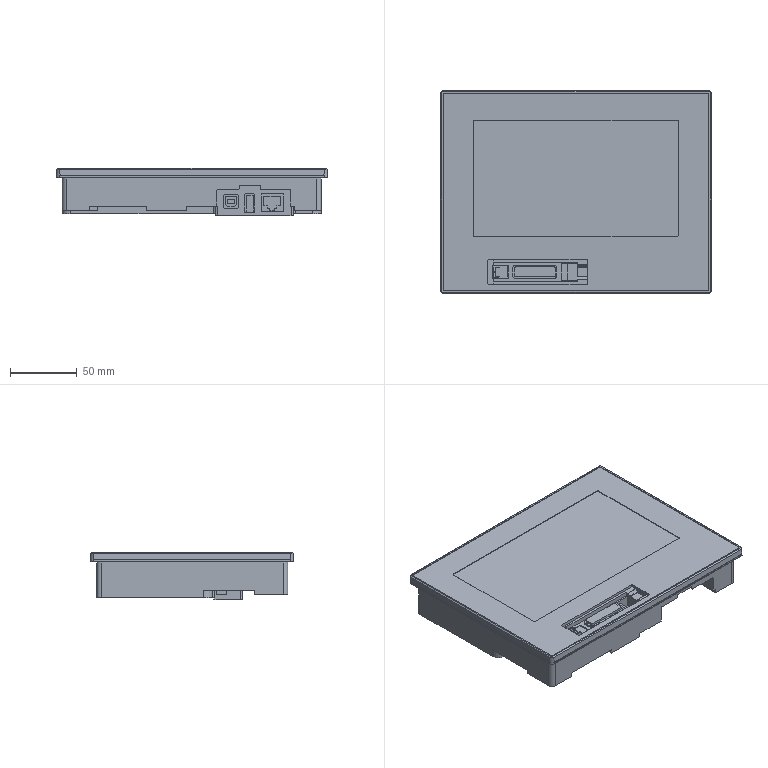Part | SolidWorks | features BaseBody 1 | 1 solid | 668 faces | box 203 x 152 x 35.35 mm | volume 852828 mm3 | plane 547 | cylinder 121 | commonest cylinder face diameters 1 x28 2 x20 2.5 x8 7 x8 3 x6 0.2 x4